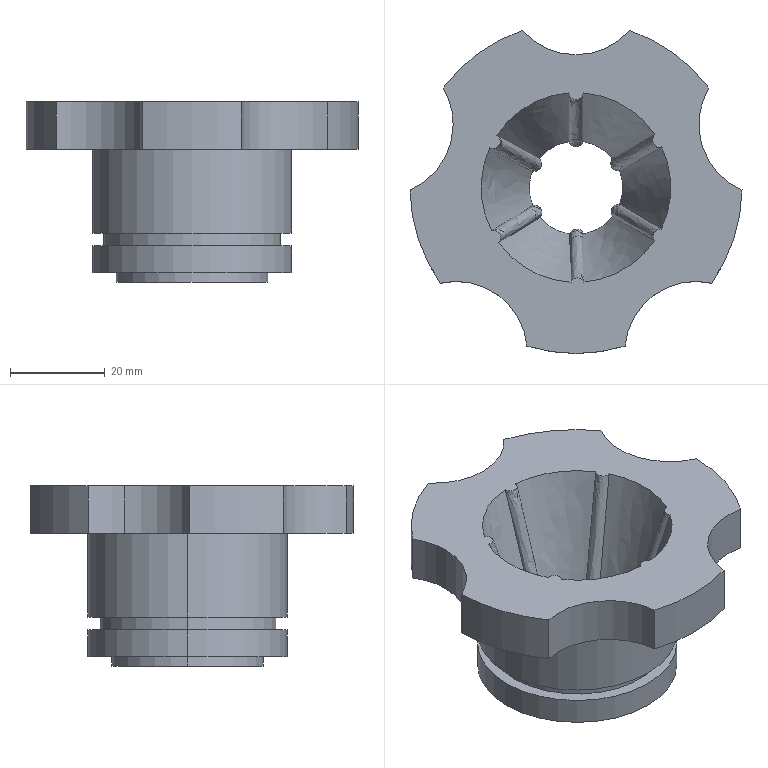Part | STEP file | Adjusting nut SGN-4-09-01 (15), threaded | 1 solid | 54 faces | box 69.993 x 68.128 x 38 mm | volume 44218 mm3 | spline 24 | cylinder 21 | plane 7 | cone 2 | commonest cylinder face diameters 30 x6 70 x5 42 x4 32 x2 37.3 x2 52 x2